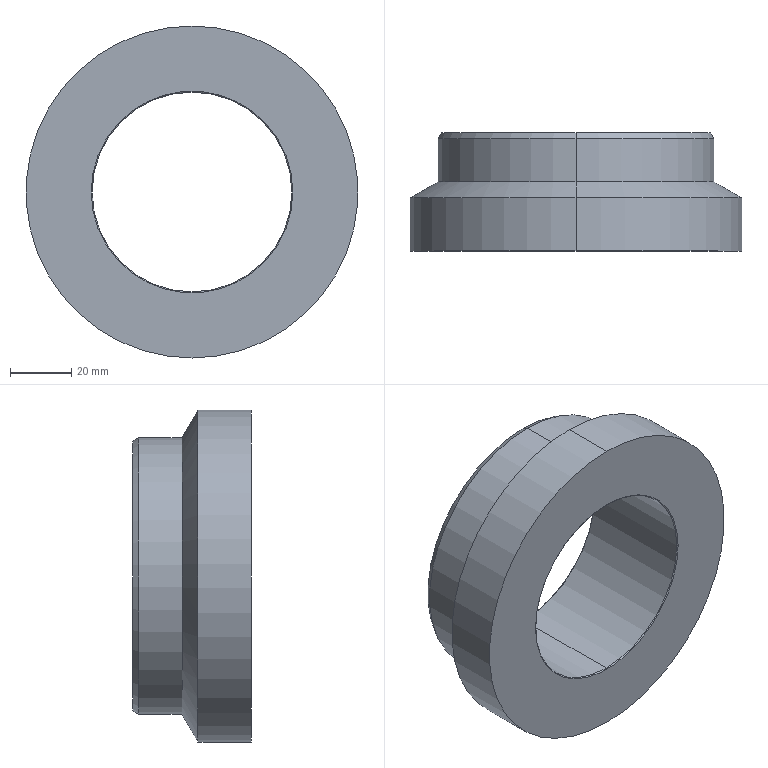Part | SolidWorks | features BaseBody 1 | 1 solid | 16 faces | box 108 x 38.5 x 108 mm | volume 172330 mm3 | cylinder 6 | cone 4 | torus 4 | plane 2 | commonest cylinder face diameters 65 x2 90 x2 108 x2
STEP:
#1=CARTESIAN_POINT('',(-2100.15,791.069,-1577.624));
#2=VERTEX_POINT('',#1);
#3=CARTESIAN_POINT('',(-2165.75,791.069,-1577.624));
#4=VERTEX_POINT('',#3);
#5=CARTESIAN_POINT('',(-2132.95,791.069,-1577.624));
#6=DIRECTION('',(0.,-1.,0.));
#7=DIRECTION('',(0.,0.,1.));
#8=AXIS2_PLACEMENT_3D('',#5,#6,#7);
#9=CIRCLE('',#8,32.8);
#10=EDGE_CURVE('',#2,#4,#9,.T.);
#11=ORIENTED_EDGE('',*,*,#10,.F.);
#12=CARTESIAN_POINT('',(-2132.95,791.069,-1577.624));
#13=DIRECTION('',(0.,-1.,0.));
#14=DIRECTION('',(-1.,0.,0.));
#15=AXIS2_PLACEMENT_3D('',#12,#13,#14);
#16=CIRCLE('',#15,32.8);
#17=EDGE_CURVE('',#4,#2,#16,.T.);
#18=ORIENTED_EDGE('',*,*,#17,.F.);
#19=EDGE_LOOP('',(#11,#18));
#20=FACE_BOUND('',#19,.T.);
#21=CARTESIAN_POINT('',(-2132.95,791.069,-1523.624));
#22=VERTEX_POINT('',#21);
#23=CARTESIAN_POINT('',(-2132.95,791.069,-1631.624));
#24=VERTEX_POINT('',#23);
#25=CARTESIAN_POINT('',(-2132.95,791.069,-1577.624));
#26=DIRECTION('',(0.,-1.,0.));
#27=DIRECTION('',(0.,0.,1.));
#28=AXIS2_PLACEMENT_3D('',#25,#26,#27);
#29=CIRCLE('',#28,54.);
#30=EDGE_CURVE('',#22,#24,#29,.T.);
#31=ORIENTED_EDGE('',*,*,#30,.T.);
#32=CARTESIAN_POINT('',(-2132.95,791.069,-1577.624));
#33=DIRECTION('',(0.,-1.,0.));
#34=DIRECTION('',(0.,0.,-1.));
#35=AXIS2_PLACEMENT_3D('',#32,#33,#34);
#36=CIRCLE('',#35,54.);
#37=EDGE_CURVE('',#24,#22,#36,.T.);
#38=ORIENTED_EDGE('',*,*,#37,.T.);
#39=EDGE_LOOP('',(#31,#38));
#40=FACE_OUTER_BOUND('',#39,.T.);
#41=CARTESIAN_POINT('',(-2073.589,791.069,-1637.024));
#42=DIRECTION('',(0.,-1.,0.));
#43=DIRECTION('',(0.,0.,-1.));
#44=AXIS2_PLACEMENT_3D('',#41,#42,#43);
#45=PLANE('',#44);
#46=ADVANCED_FACE('',(#20,#40),#45,.T.);
#47=CARTESIAN_POINT('',(-2132.95,808.372,-1523.624));
#48=VERTEX_POINT('',#47);
#49=CARTESIAN_POINT('',(-2132.95,808.372,-1523.624));
#50=DIRECTION('',(0.,-1.,0.));
#51=VECTOR('',#50,1000.);
#52=LINE('',#49,#51);
#53=EDGE_CURVE('',#48,#22,#52,.T.);
#54=ORIENTED_EDGE('',*,*,#53,.T.);
#55=ORIENTED_EDGE('',*,*,#37,.F.);
#56=CARTESIAN_POINT('',(-2132.95,808.372,-1631.624));
#57=VERTEX_POINT('',#56);
#58=CARTESIAN_POINT('',(-2132.95,791.069,-1631.624));
#59=DIRECTION('',(0.,1.,0.));
#60=VECTOR('',#59,1000.);
#61=LINE('',#58,#60);
#62=EDGE_CURVE('',#24,#57,#61,.T.);
#63=ORIENTED_EDGE('',*,*,#62,.T.);
#64=CARTESIAN_POINT('',(-2132.95,808.372,-1577.624));
#65=DIRECTION('',(0.,-1.,0.));
#66=DIRECTION('',(0.,0.,-1.));
#67=AXIS2_PLACEMENT_3D('',#64,#65,#66);
#68=CIRCLE('',#67,54.);
#69=EDGE_CURVE('',#57,#48,#68,.T.);
#70=ORIENTED_EDGE('',*,*,#69,.T.);
#71=EDGE_LOOP('',(#54,#55,#63,#70));
#72=FACE_OUTER_BOUND('',#71,.T.);
#73=CARTESIAN_POINT('',(-2132.95,809.238,-1577.624));
#74=DIRECTION('',(0.,1.,0.));
#75=DIRECTION('',(-0.08716,0.,0.9962));
#76=AXIS2_PLACEMENT_3D('',#73,#74,#75);
#77=CYLINDRICAL_SURFACE('',#76,54.);
#78=ADVANCED_FACE('',(#72),#77,.T.);
#79=CARTESIAN_POINT('',(-2132.95,813.569,-1532.624));
#80=VERTEX_POINT('',#79);
#81=CARTESIAN_POINT('',(-2132.95,813.569,-1532.624));
#82=DIRECTION('',(0.,-0.5,0.866));
#83=VECTOR('',#82,1000.);
#84=LINE('',#81,#83);
#85=EDGE_CURVE('',#80,#48,#84,.T.);
#86=ORIENTED_EDGE('',*,*,#85,.T.);
#87=ORIENTED_EDGE('',*,*,#69,.F.);
#88=CARTESIAN_POINT('',(-2132.95,813.569,-1622.624));
#89=VERTEX_POINT('',#88);
#90=CARTESIAN_POINT('',(-2132.95,808.372,-1631.624));
#91=DIRECTION('',(0.,0.5,0.866));
#92=VECTOR('',#91,1000.);
#93=LINE('',#90,#92);
#94=EDGE_CURVE('',#57,#89,#93,.T.);
#95=ORIENTED_EDGE('',*,*,#94,.T.);
#96=CARTESIAN_POINT('',(-2132.95,813.569,-1577.624));
#97=DIRECTION('',(0.,-1.,0.));
#98=DIRECTION('',(0.,0.,-1.));
#99=AXIS2_PLACEMENT_3D('',#96,#97,#98);
#100=CIRCLE('',#99,45.);
#101=EDGE_CURVE('',#89,#80,#100,.T.);
#102=ORIENTED_EDGE('',*,*,#101,.T.);
#103=EDGE_LOOP('',(#86,#87,#95,#102));
#104=FACE_OUTER_BOUND('',#103,.T.);
#105=CARTESIAN_POINT('',(-2132.95,813.828,-1577.624));
#106=DIRECTION('',(0.,-1.,0.));
#107=DIRECTION('',(-0.08716,0.,-0.9962));
#108=AXIS2_PLACEMENT_3D('',#105,#106,#107);
#109=CONICAL_SURFACE('',#108,44.55,1.047);
#110=ADVANCED_FACE('',(#104),#109,.T.);
#111=CARTESIAN_POINT('',(-2132.95,827.569,-1532.624));
#112=VERTEX_POINT('',#111);
#113=CARTESIAN_POINT('',(-2132.95,827.569,-1532.624));
#114=DIRECTION('',(0.,-1.,0.));
#115=VECTOR('',#114,1000.);
#116=LINE('',#113,#115);
#117=EDGE_CURVE('',#112,#80,#116,.T.);
#118=ORIENTED_EDGE('',*,*,#117,.T.);
#119=ORIENTED_EDGE('',*,*,#101,.F.);
#120=CARTESIAN_POINT('',(-2132.95,827.569,-1622.624));
#121=VERTEX_POINT('',#120);
#122=CARTESIAN_POINT('',(-2132.95,813.569,-1622.624));
#123=DIRECTION('',(0.,1.,0.));
#124=VECTOR('',#123,1000.);
#125=LINE('',#122,#124);
#126=EDGE_CURVE('',#89,#121,#125,.T.);
#127=ORIENTED_EDGE('',*,*,#126,.T.);
#128=CARTESIAN_POINT('',(-2132.95,827.569,-1577.624));
#129=DIRECTION('',(0.,-1.,0.));
#130=DIRECTION('',(0.,0.,-1.));
#131=AXIS2_PLACEMENT_3D('',#128,#129,#130);
#132=CIRCLE('',#131,45.);
#133=EDGE_CURVE('',#121,#112,#132,.T.);
#134=ORIENTED_EDGE('',*,*,#133,.T.);
#135=EDGE_LOOP('',(#118,#119,#127,#134));
#136=FACE_OUTER_BOUND('',#135,.T.);
#137=CARTESIAN_POINT('',(-2132.95,828.269,-1577.624));
#138=DIRECTION('',(0.,1.,0.));
#139=DIRECTION('',(-0.08716,0.,0.9962));
#140=AXIS2_PLACEMENT_3D('',#137,#138,#139);
#141=CYLINDRICAL_SURFACE('',#140,45.);
#142=ADVANCED_FACE('',(#136),#141,.T.);
#143=CARTESIAN_POINT('',(-2132.95,829.569,-1533.774));
#144=VERTEX_POINT('',#143);
#145=CARTESIAN_POINT('',(-2132.95,829.569,-1533.774));
#146=DIRECTION('',(0.,-0.8669,0.4985));
#147=VECTOR('',#146,1000.);
#148=LINE('',#145,#147);
#149=EDGE_CURVE('',#144,#112,#148,.T.);
#150=ORIENTED_EDGE('',*,*,#149,.T.);
#151=ORIENTED_EDGE('',*,*,#133,.F.);
#152=CARTESIAN_POINT('',(-2132.95,829.569,-1621.474));
#153=VERTEX_POINT('',#152);
#154=CARTESIAN_POINT('',(-2132.95,827.569,-1622.624));
#155=DIRECTION('',(0.,0.8669,0.4985));
#156=VECTOR('',#155,1000.);
#157=LINE('',#154,#156);
#158=EDGE_CURVE('',#121,#153,#157,.T.);
#159=ORIENTED_EDGE('',*,*,#158,.T.);
#160=CARTESIAN_POINT('',(-2132.95,829.569,-1577.624));
#161=DIRECTION('',(0.,1.,0.));
#162=DIRECTION('',(0.,0.,1.));
#163=AXIS2_PLACEMENT_3D('',#160,#161,#162);
#164=CIRCLE('',#163,43.85);
#165=EDGE_CURVE('',#144,#153,#164,.T.);
#166=ORIENTED_EDGE('',*,*,#165,.F.);
#167=EDGE_LOOP('',(#150,#151,#159,#166));
#168=FACE_OUTER_BOUND('',#167,.T.);
#169=CARTESIAN_POINT('',(-2132.95,829.669,-1577.624));
#170=DIRECTION('',(0.,-1.,0.));
#171=DIRECTION('',(-0.08716,0.,-0.9962));
#172=AXIS2_PLACEMENT_3D('',#169,#170,#171);
#173=CONICAL_SURFACE('',#172,43.792,0.5218);
#174=ADVANCED_FACE('',(#168),#173,.T.);
#175=CARTESIAN_POINT('',(-2165.75,829.569,-1577.624));
#176=VERTEX_POINT('',#175);
#177=CARTESIAN_POINT('',(-2100.15,829.569,-1577.624));
#178=VERTEX_POINT('',#177);
#179=CARTESIAN_POINT('',(-2132.95,829.569,-1577.624));
#180=DIRECTION('',(0.,1.,0.));
#181=DIRECTION('',(-1.,0.,0.));
#182=AXIS2_PLACEMENT_3D('',#179,#180,#181);
#183=CIRCLE('',#182,32.8);
#184=EDGE_CURVE('',#176,#178,#183,.T.);
#185=ORIENTED_EDGE('',*,*,#184,.F.);
#186=CARTESIAN_POINT('',(-2132.95,829.569,-1577.624));
#187=DIRECTION('',(0.,1.,0.));
#188=DIRECTION('',(1.,0.,0.));
#189=AXIS2_PLACEMENT_3D('',#186,#187,#188);
#190=CIRCLE('',#189,32.8);
#191=EDGE_CURVE('',#178,#176,#190,.T.);
#192=ORIENTED_EDGE('',*,*,#191,.F.);
#193=EDGE_LOOP('',(#185,#192));
#194=FACE_BOUND('',#193,.T.);
#195=CARTESIAN_POINT('',(-2132.95,829.569,-1577.624));
#196=DIRECTION('',(0.,1.,0.));
#197=DIRECTION('',(0.,0.,-1.));
#198=AXIS2_PLACEMENT_3D('',#195,#196,#197);
#199=CIRCLE('',#198,43.85);
#200=EDGE_CURVE('',#153,#144,#199,.T.);
#201=ORIENTED_EDGE('',*,*,#200,.T.);
#202=ORIENTED_EDGE('',*,*,#165,.T.);
#203=EDGE_LOOP('',(#201,#202));
#204=FACE_OUTER_BOUND('',#203,.T.);
#205=CARTESIAN_POINT('',(-2084.754,829.569,-1529.389));
#206=DIRECTION('',(0.,1.,0.));
#207=DIRECTION('',(1.,0.,0.));
#208=AXIS2_PLACEMENT_3D('',#205,#206,#207);
#209=PLANE('',#208);
#210=ADVANCED_FACE('',(#194,#204),#209,.T.);
#211=CARTESIAN_POINT('',(-2100.45,829.269,-1577.624));
#212=VERTEX_POINT('',#211);
#213=CARTESIAN_POINT('',(-2100.15,829.269,-1577.624));
#214=DIRECTION('',(0.,0.,-1.));
#215=DIRECTION('',(-1.,0.,0.));
#216=AXIS2_PLACEMENT_3D('',#213,#214,#215);
#217=CIRCLE('',#216,0.3);
#218=EDGE_CURVE('',#212,#178,#217,.T.);
#219=ORIENTED_EDGE('',*,*,#218,.T.);
#220=ORIENTED_EDGE('',*,*,#191,.T.);
#221=CARTESIAN_POINT('',(-2165.45,829.269,-1577.624));
#222=VERTEX_POINT('',#221);
#223=CARTESIAN_POINT('',(-2165.75,829.269,-1577.624));
#224=DIRECTION('',(0.,0.,-1.));
#225=DIRECTION('',(0.,1.,0.));
#226=AXIS2_PLACEMENT_3D('',#223,#224,#225);
#227=CIRCLE('',#226,0.3);
#228=EDGE_CURVE('',#176,#222,#227,.T.);
#229=ORIENTED_EDGE('',*,*,#228,.T.);
#230=CARTESIAN_POINT('',(-2132.95,829.269,-1610.124));
#231=VERTEX_POINT('',#230);
#232=CARTESIAN_POINT('',(-2132.95,829.269,-1577.624));
#233=DIRECTION('',(0.,-1.,0.));
#234=DIRECTION('',(-1.,0.,0.));
#235=AXIS2_PLACEMENT_3D('',#232,#233,#234);
#236=CIRCLE('',#235,32.5);
#237=EDGE_CURVE('',#222,#231,#236,.T.);
#238=ORIENTED_EDGE('',*,*,#237,.T.);
#239=CARTESIAN_POINT('',(-2132.95,829.269,-1577.624));
#240=DIRECTION('',(0.,-1.,0.));
#241=DIRECTION('',(0.,0.,-1.));
#242=AXIS2_PLACEMENT_3D('',#239,#240,#241);
#243=CIRCLE('',#242,32.5);
#244=EDGE_CURVE('',#231,#212,#243,.T.);
#245=ORIENTED_EDGE('',*,*,#244,.T.);
#246=EDGE_LOOP('',(#219,#220,#229,#238,#245));
#247=FACE_OUTER_BOUND('',#246,.T.);
#248=CARTESIAN_POINT('',(-2132.95,829.269,-1577.624));
#249=DIRECTION('',(0.,-1.,0.));
#250=DIRECTION('',(-0.9962,0.,0.08716));
#251=AXIS2_PLACEMENT_3D('',#248,#249,#250);
#252=TOROIDAL_SURFACE('',#251,32.8,0.3);
#253=ADVANCED_FACE('',(#247),#252,.T.);
#254=CARTESIAN_POINT('',(-2132.95,829.269,-1545.124));
#255=VERTEX_POINT('',#254);
#256=CARTESIAN_POINT('',(-2132.95,791.369,-1545.124));
#257=VERTEX_POINT('',#256);
#258=CARTESIAN_POINT('',(-2132.95,829.269,-1545.124));
#259=DIRECTION('',(0.,-1.,0.));
#260=VECTOR('',#259,1000.);
#261=LINE('',#258,#260);
#262=EDGE_CURVE('',#255,#257,#261,.T.);
#263=ORIENTED_EDGE('',*,*,#262,.T.);
#264=CARTESIAN_POINT('',(-2165.45,791.369,-1577.624));
#265=VERTEX_POINT('',#264);
#266=CARTESIAN_POINT('',(-2132.95,791.369,-1577.624));
#267=DIRECTION('',(0.,-1.,0.));
#268=DIRECTION('',(0.,0.,1.));
#269=AXIS2_PLACEMENT_3D('',#266,#267,#268);
#270=CIRCLE('',#269,32.5);
#271=EDGE_CURVE('',#257,#265,#270,.T.);
#272=ORIENTED_EDGE('',*,*,#271,.T.);
#273=CARTESIAN_POINT('',(-2132.95,791.369,-1610.124));
#274=VERTEX_POINT('',#273);
#275=CARTESIAN_POINT('',(-2132.95,791.369,-1577.624));
#276=DIRECTION('',(0.,-1.,0.));
#277=DIRECTION('',(-1.,0.,0.));
#278=AXIS2_PLACEMENT_3D('',#275,#276,#277);
#279=CIRCLE('',#278,32.5);
#280=EDGE_CURVE('',#265,#274,#279,.T.);
#281=ORIENTED_EDGE('',*,*,#280,.T.);
#282=CARTESIAN_POINT('',(-2132.95,791.369,-1610.124));
#283=DIRECTION('',(0.,1.,0.));
#284=VECTOR('',#283,1000.);
#285=LINE('',#282,#284);
#286=EDGE_CURVE('',#274,#231,#285,.T.);
#287=ORIENTED_EDGE('',*,*,#286,.T.);
#288=ORIENTED_EDGE('',*,*,#237,.F.);
#289=CARTESIAN_POINT('',(-2132.95,829.269,-1577.624));
#290=DIRECTION('',(0.,-1.,0.));
#291=DIRECTION('',(0.,0.,1.));
#292=AXIS2_PLACEMENT_3D('',#289,#290,#291);
#293=CIRCLE('',#292,32.5);
#294=EDGE_CURVE('',#255,#222,#293,.T.);
#295=ORIENTED_EDGE('',*,*,#294,.F.);
#296=EDGE_LOOP('',(#263,#272,#281,#287,#288,#295));
#297=FACE_OUTER_BOUND('',#296,.T.);
#298=CARTESIAN_POINT('',(-2132.95,789.474,-1577.624));
#299=DIRECTION('',(0.,1.,0.));
#300=DIRECTION('',(0.08716,0.,-0.9962));
#301=AXIS2_PLACEMENT_3D('',#298,#299,#300);
#302=CYLINDRICAL_SURFACE('',#301,32.5);
#303=ADVANCED_FACE('',(#297),#302,.F.);
#304=CARTESIAN_POINT('',(-2100.45,791.369,-1577.624));
#305=VERTEX_POINT('',#304);
#306=CARTESIAN_POINT('',(-2100.15,791.369,-1577.624));
#307=DIRECTION('',(0.,0.,-1.));
#308=DIRECTION('',(0.,-1.,0.));
#309=AXIS2_PLACEMENT_3D('',#306,#307,#308);
#310=CIRCLE('',#309,0.3);
#311=EDGE_CURVE('',#2,#305,#310,.T.);
#312=ORIENTED_EDGE('',*,*,#311,.T.);
#313=CARTESIAN_POINT('',(-2132.95,791.369,-1577.624));
#314=DIRECTION('',(0.,-1.,0.));
#315=DIRECTION('',(0.,0.,-1.));
#316=AXIS2_PLACEMENT_3D('',#313,#314,#315);
#317=CIRCLE('',#316,32.5);
#318=EDGE_CURVE('',#274,#305,#317,.T.);
#319=ORIENTED_EDGE('',*,*,#318,.F.);
#320=ORIENTED_EDGE('',*,*,#280,.F.);
#321=CARTESIAN_POINT('',(-2165.75,791.369,-1577.624));
#322=DIRECTION('',(0.,0.,-1.));
#323=DIRECTION('',(1.,0.,0.));
#324=AXIS2_PLACEMENT_3D('',#321,#322,#323);
#325=CIRCLE('',#324,0.3);
#326=EDGE_CURVE('',#265,#4,#325,.T.);
#327=ORIENTED_EDGE('',*,*,#326,.T.);
#328=ORIENTED_EDGE('',*,*,#17,.T.);
#329=EDGE_LOOP('',(#312,#319,#320,#327,#328));
#330=FACE_OUTER_BOUND('',#329,.T.);
#331=CARTESIAN_POINT('',(-2132.95,791.369,-1577.624));
#332=DIRECTION('',(0.,-1.,0.));
#333=DIRECTION('',(-0.9962,0.,0.08716));
#334=AXIS2_PLACEMENT_3D('',#331,#332,#333);
#335=TOROIDAL_SURFACE('',#334,32.8,0.3);
#336=ADVANCED_FACE('',(#330),#335,.T.);
#337=ORIENTED_EDGE('',*,*,#311,.F.);
#338=ORIENTED_EDGE('',*,*,#10,.T.);
#339=ORIENTED_EDGE('',*,*,#326,.F.);
#340=ORIENTED_EDGE('',*,*,#271,.F.);
#341=CARTESIAN_POINT('',(-2132.95,791.369,-1577.624));
#342=DIRECTION('',(0.,-1.,0.));
#343=DIRECTION('',(1.,0.,0.));
#344=AXIS2_PLACEMENT_3D('',#341,#342,#343);
#345=CIRCLE('',#344,32.5);
#346=EDGE_CURVE('',#305,#257,#345,.T.);
#347=ORIENTED_EDGE('',*,*,#346,.F.);
#348=EDGE_LOOP('',(#337,#338,#339,#340,#347));
#349=FACE_OUTER_BOUND('',#348,.T.);
#350=CARTESIAN_POINT('',(-2132.95,791.369,-1577.624));
#351=DIRECTION('',(0.,-1.,0.));
#352=DIRECTION('',(0.9962,0.,-0.08716));
#353=AXIS2_PLACEMENT_3D('',#350,#351,#352);
#354=TOROIDAL_SURFACE('',#353,32.8,0.3);
#355=ADVANCED_FACE('',(#349),#354,.T.);
#356=ORIENTED_EDGE('',*,*,#262,.F.);
#357=CARTESIAN_POINT('',(-2132.95,829.269,-1577.624));
#358=DIRECTION('',(0.,-1.,0.));
#359=DIRECTION('',(1.,0.,0.));
#360=AXIS2_PLACEMENT_3D('',#357,#358,#359);
#361=CIRCLE('',#360,32.5);
#362=EDGE_CURVE('',#212,#255,#361,.T.);
#363=ORIENTED_EDGE('',*,*,#362,.F.);
#364=ORIENTED_EDGE('',*,*,#244,.F.);
#365=ORIENTED_EDGE('',*,*,#286,.F.);
#366=ORIENTED_EDGE('',*,*,#318,.T.);
#367=ORIENTED_EDGE('',*,*,#346,.T.);
#368=EDGE_LOOP('',(#356,#363,#364,#365,#366,#367));
#369=FACE_OUTER_BOUND('',#368,.T.);
#370=CARTESIAN_POINT('',(-2132.95,789.474,-1577.624));
#371=DIRECTION('',(0.,1.,0.));
#372=DIRECTION('',(-0.08716,0.,0.9962));
#373=AXIS2_PLACEMENT_3D('',#370,#371,#372);
#374=CYLINDRICAL_SURFACE('',#373,32.5);
#375=ADVANCED_FACE('',(#369),#374,.F.);
#376=ORIENTED_EDGE('',*,*,#218,.F.);
#377=ORIENTED_EDGE('',*,*,#362,.T.);
#378=ORIENTED_EDGE('',*,*,#294,.T.);
#379=ORIENTED_EDGE('',*,*,#228,.F.);
#380=ORIENTED_EDGE('',*,*,#184,.T.);
#381=EDGE_LOOP('',(#376,#377,#378,#379,#380));
#382=FACE_OUTER_BOUND('',#381,.T.);
#383=CARTESIAN_POINT('',(-2132.95,829.269,-1577.624));
#384=DIRECTION('',(0.,-1.,0.));
#385=DIRECTION('',(0.9962,0.,-0.08716));
#386=AXIS2_PLACEMENT_3D('',#383,#384,#385);
#387=TOROIDAL_SURFACE('',#386,32.8,0.3);
#388=ADVANCED_FACE('',(#382),#387,.T.);
#389=ORIENTED_EDGE('',*,*,#149,.F.);
#390=ORIENTED_EDGE('',*,*,#200,.F.);
#391=ORIENTED_EDGE('',*,*,#158,.F.);
#392=CARTESIAN_POINT('',(-2132.95,827.569,-1577.624));
#393=DIRECTION('',(0.,-1.,0.));
#394=DIRECTION('',(0.,0.,1.));
#395=AXIS2_PLACEMENT_3D('',#392,#393,#394);
#396=CIRCLE('',#395,45.);
#397=EDGE_CURVE('',#112,#121,#396,.T.);
#398=ORIENTED_EDGE('',*,*,#397,.F.);
#399=EDGE_LOOP('',(#389,#390,#391,#398));
#400=FACE_OUTER_BOUND('',#399,.T.);
#401=CARTESIAN_POINT('',(-2132.95,829.669,-1577.624));
#402=DIRECTION('',(0.,-1.,0.));
#403=DIRECTION('',(0.08716,0.,0.9962));
#404=AXIS2_PLACEMENT_3D('',#401,#402,#403);
#405=CONICAL_SURFACE('',#404,43.792,0.5218);
#406=ADVANCED_FACE('',(#400),#405,.T.);
#407=ORIENTED_EDGE('',*,*,#117,.F.);
#408=ORIENTED_EDGE('',*,*,#397,.T.);
#409=ORIENTED_EDGE('',*,*,#126,.F.);
#410=CARTESIAN_POINT('',(-2132.95,813.569,-1577.624));
#411=DIRECTION('',(0.,-1.,0.));
#412=DIRECTION('',(0.,0.,1.));
#413=AXIS2_PLACEMENT_3D('',#410,#411,#412);
#414=CIRCLE('',#413,45.);
#415=EDGE_CURVE('',#80,#89,#414,.T.);
#416=ORIENTED_EDGE('',*,*,#415,.F.);
#417=EDGE_LOOP('',(#407,#408,#409,#416));
#418=FACE_OUTER_BOUND('',#417,.T.);
#419=CARTESIAN_POINT('',(-2132.95,828.269,-1577.624));
#420=DIRECTION('',(0.,1.,0.));
#421=DIRECTION('',(0.08716,0.,-0.9962));
#422=AXIS2_PLACEMENT_3D('',#419,#420,#421);
#423=CYLINDRICAL_SURFACE('',#422,45.);
#424=ADVANCED_FACE('',(#418),#423,.T.);
#425=ORIENTED_EDGE('',*,*,#85,.F.);
#426=ORIENTED_EDGE('',*,*,#415,.T.);
#427=ORIENTED_EDGE('',*,*,#94,.F.);
#428=CARTESIAN_POINT('',(-2132.95,808.372,-1577.624));
#429=DIRECTION('',(0.,-1.,0.));
#430=DIRECTION('',(0.,0.,1.));
#431=AXIS2_PLACEMENT_3D('',#428,#429,#430);
#432=CIRCLE('',#431,54.);
#433=EDGE_CURVE('',#48,#57,#432,.T.);
#434=ORIENTED_EDGE('',*,*,#433,.F.);
#435=EDGE_LOOP('',(#425,#426,#427,#434));
#436=FACE_OUTER_BOUND('',#435,.T.);
#437=CARTESIAN_POINT('',(-2132.95,813.828,-1577.624));
#438=DIRECTION('',(0.,-1.,0.));
#439=DIRECTION('',(0.08716,0.,0.9962));
#440=AXIS2_PLACEMENT_3D('',#437,#438,#439);
#441=CONICAL_SURFACE('',#440,44.55,1.047);
#442=ADVANCED_FACE('',(#436),#441,.T.);
#443=ORIENTED_EDGE('',*,*,#53,.F.);
#444=ORIENTED_EDGE('',*,*,#433,.T.);
#445=ORIENTED_EDGE('',*,*,#62,.F.);
#446=ORIENTED_EDGE('',*,*,#30,.F.);
#447=EDGE_LOOP('',(#443,#444,#445,#446));
#448=FACE_OUTER_BOUND('',#447,.T.);
#449=CARTESIAN_POINT('',(-2132.95,809.238,-1577.624));
#450=DIRECTION('',(0.,1.,0.));
#451=DIRECTION('',(0.08716,0.,-0.9962));
#452=AXIS2_PLACEMENT_3D('',#449,#450,#451);
#453=CYLINDRICAL_SURFACE('',#452,54.);
#454=ADVANCED_FACE('',(#448),#453,.T.);
#455=CLOSED_SHELL('',(#46,#78,#110,#142,#174,#210,#253,#303,#336,#355,#375,#388,#406,#424,#442,#454));
#456=MANIFOLD_SOLID_BREP('',#455);
#457=CARTESIAN_POINT('',(0.,0.,0.));
#458=DIRECTION('',(0.,0.,1.));
#459=DIRECTION('',(1.,0.,0.));
#460=AXIS2_PLACEMENT_3D('',#457,#458,#459);
#461=(LENGTH_UNIT()NAMED_UNIT(*)SI_UNIT(.MILLI.,.METRE.));
#462=UNCERTAINTY_MEASURE_WITH_UNIT(LENGTH_MEASURE(0.00001),#461,'','');
#463=(NAMED_UNIT(*)PLANE_ANGLE_UNIT()SI_UNIT($,.RADIAN.));
#464=(NAMED_UNIT(*)SI_UNIT($,.STERADIAN.)SOLID_ANGLE_UNIT());
#465=(GEOMETRIC_REPRESENTATION_CONTEXT(3)GLOBAL_UNCERTAINTY_ASSIGNED_CONTEXT((#462))GLOBAL_UNIT_ASSIGNED_CONTEXT((#461,#463,#464))REPRESENTATION_CONTEXT('',''));
#466=ADVANCED_BREP_SHAPE_REPRESENTATION('',(#456,#460),#465);